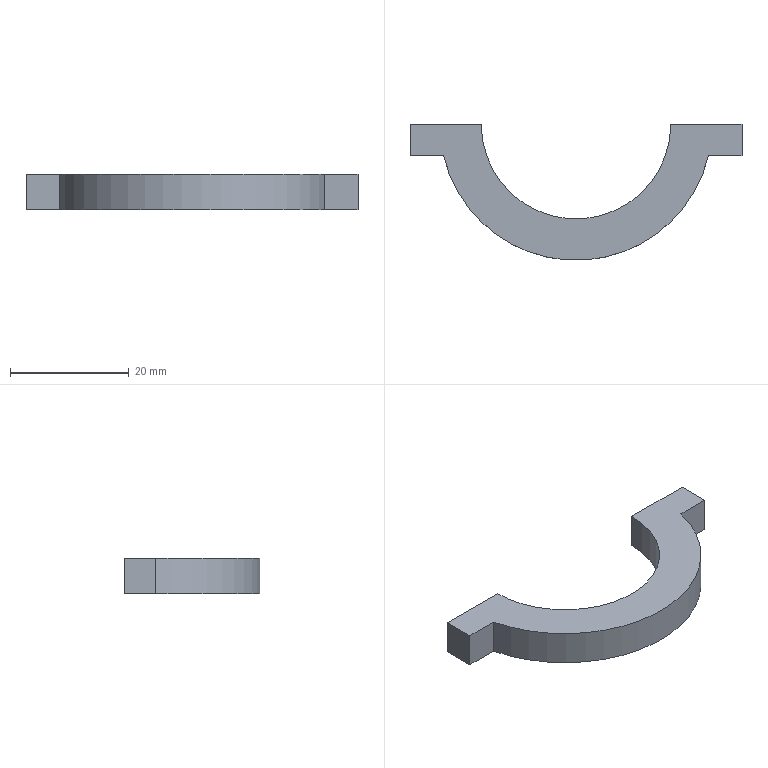Part | SolidWorks | features Extrusion 1 | 1 solid | 10 faces | box 56 x 22.979 x 6 mm | volume 2901 mm3 | plane 8 | cylinder 2 | commonest cylinder face diameters 32 x1 45.958 x1
STEP:
#1=CARTESIAN_POINT('',(16.,50.,0.));
#2=VERTEX_POINT('',#1);
#3=CARTESIAN_POINT('',(-16.,50.,0.));
#4=VERTEX_POINT('',#3);
#5=CARTESIAN_POINT('',(0.,50.,0.));
#6=DIRECTION('',(0.,0.,-1.));
#7=DIRECTION('',(1.,0.,0.));
#8=AXIS2_PLACEMENT_3D('',#5,#6,#7);
#9=CIRCLE('',#8,16.);
#10=EDGE_CURVE('',#2,#4,#9,.T.);
#11=ORIENTED_EDGE('',*,*,#10,.T.);
#12=CARTESIAN_POINT('',(-16.,50.,6.));
#13=VERTEX_POINT('',#12);
#14=CARTESIAN_POINT('',(-16.,50.,6.));
#15=DIRECTION('',(0.,0.,-1.));
#16=VECTOR('',#15,1000.);
#17=LINE('',#14,#16);
#18=EDGE_CURVE('',#13,#4,#17,.T.);
#19=ORIENTED_EDGE('',*,*,#18,.F.);
#20=CARTESIAN_POINT('',(16.,50.,6.));
#21=VERTEX_POINT('',#20);
#22=CARTESIAN_POINT('',(0.,50.,6.));
#23=DIRECTION('',(0.,0.,-1.));
#24=DIRECTION('',(1.,0.,0.));
#25=AXIS2_PLACEMENT_3D('',#22,#23,#24);
#26=CIRCLE('',#25,16.);
#27=EDGE_CURVE('',#21,#13,#26,.T.);
#28=ORIENTED_EDGE('',*,*,#27,.F.);
#29=CARTESIAN_POINT('',(16.,50.,6.));
#30=DIRECTION('',(0.,0.,-1.));
#31=VECTOR('',#30,1000.);
#32=LINE('',#29,#31);
#33=EDGE_CURVE('',#21,#2,#32,.T.);
#34=ORIENTED_EDGE('',*,*,#33,.T.);
#35=EDGE_LOOP('',(#11,#19,#28,#34));
#36=FACE_OUTER_BOUND('',#35,.T.);
#37=CARTESIAN_POINT('',(0.,50.,6.));
#38=DIRECTION('',(0.,0.,-1.));
#39=DIRECTION('',(-1.,0.,0.));
#40=AXIS2_PLACEMENT_3D('',#37,#38,#39);
#41=CYLINDRICAL_SURFACE('',#40,16.);
#42=ADVANCED_FACE('',(#36),#41,.F.);
#43=CARTESIAN_POINT('',(-28.,50.,0.));
#44=VERTEX_POINT('',#43);
#45=CARTESIAN_POINT('',(-16.,50.,0.));
#46=DIRECTION('',(-1.,0.,0.));
#47=VECTOR('',#46,1000.);
#48=LINE('',#45,#47);
#49=EDGE_CURVE('',#4,#44,#48,.T.);
#50=ORIENTED_EDGE('',*,*,#49,.T.);
#51=CARTESIAN_POINT('',(-28.,50.,6.));
#52=VERTEX_POINT('',#51);
#53=CARTESIAN_POINT('',(-28.,50.,6.));
#54=DIRECTION('',(0.,0.,-1.));
#55=VECTOR('',#54,1000.);
#56=LINE('',#53,#55);
#57=EDGE_CURVE('',#52,#44,#56,.T.);
#58=ORIENTED_EDGE('',*,*,#57,.F.);
#59=CARTESIAN_POINT('',(-16.,50.,6.));
#60=DIRECTION('',(-1.,0.,0.));
#61=VECTOR('',#60,1000.);
#62=LINE('',#59,#61);
#63=EDGE_CURVE('',#13,#52,#62,.T.);
#64=ORIENTED_EDGE('',*,*,#63,.F.);
#65=ORIENTED_EDGE('',*,*,#18,.T.);
#66=EDGE_LOOP('',(#50,#58,#64,#65));
#67=FACE_OUTER_BOUND('',#66,.T.);
#68=CARTESIAN_POINT('',(-16.,50.,6.));
#69=DIRECTION('',(0.,-1.,0.));
#70=DIRECTION('',(0.,0.,-1.));
#71=AXIS2_PLACEMENT_3D('',#68,#69,#70);
#72=PLANE('',#71);
#73=ADVANCED_FACE('',(#67),#72,.F.);
#74=CARTESIAN_POINT('',(-28.,44.637,0.));
#75=VERTEX_POINT('',#74);
#76=CARTESIAN_POINT('',(-28.,50.,0.));
#77=DIRECTION('',(0.,-1.,0.));
#78=VECTOR('',#77,1000.);
#79=LINE('',#76,#78);
#80=EDGE_CURVE('',#44,#75,#79,.T.);
#81=ORIENTED_EDGE('',*,*,#80,.T.);
#82=CARTESIAN_POINT('',(-28.,44.637,6.));
#83=VERTEX_POINT('',#82);
#84=CARTESIAN_POINT('',(-28.,44.637,6.));
#85=DIRECTION('',(0.,0.,-1.));
#86=VECTOR('',#85,1000.);
#87=LINE('',#84,#86);
#88=EDGE_CURVE('',#83,#75,#87,.T.);
#89=ORIENTED_EDGE('',*,*,#88,.F.);
#90=CARTESIAN_POINT('',(-28.,50.,6.));
#91=DIRECTION('',(0.,-1.,0.));
#92=VECTOR('',#91,1000.);
#93=LINE('',#90,#92);
#94=EDGE_CURVE('',#52,#83,#93,.T.);
#95=ORIENTED_EDGE('',*,*,#94,.F.);
#96=ORIENTED_EDGE('',*,*,#57,.T.);
#97=EDGE_LOOP('',(#81,#89,#95,#96));
#98=FACE_OUTER_BOUND('',#97,.T.);
#99=CARTESIAN_POINT('',(-28.,50.,6.));
#100=DIRECTION('',(1.,0.,0.));
#101=DIRECTION('',(0.,0.,-1.));
#102=AXIS2_PLACEMENT_3D('',#99,#100,#101);
#103=PLANE('',#102);
#104=ADVANCED_FACE('',(#98),#103,.F.);
#105=CARTESIAN_POINT('',(-22.345,44.637,0.));
#106=VERTEX_POINT('',#105);
#107=CARTESIAN_POINT('',(-22.345,44.637,0.));
#108=DIRECTION('',(1.,0.,0.));
#109=VECTOR('',#108,1000.);
#110=LINE('',#107,#109);
#111=EDGE_CURVE('',#75,#106,#110,.T.);
#112=ORIENTED_EDGE('',*,*,#111,.T.);
#113=CARTESIAN_POINT('',(-22.345,44.637,6.));
#114=VERTEX_POINT('',#113);
#115=CARTESIAN_POINT('',(-22.345,44.637,6.));
#116=DIRECTION('',(0.,0.,-1.));
#117=VECTOR('',#116,1000.);
#118=LINE('',#115,#117);
#119=EDGE_CURVE('',#114,#106,#118,.T.);
#120=ORIENTED_EDGE('',*,*,#119,.F.);
#121=CARTESIAN_POINT('',(-22.345,44.637,6.));
#122=DIRECTION('',(1.,0.,0.));
#123=VECTOR('',#122,1000.);
#124=LINE('',#121,#123);
#125=EDGE_CURVE('',#83,#114,#124,.T.);
#126=ORIENTED_EDGE('',*,*,#125,.F.);
#127=ORIENTED_EDGE('',*,*,#88,.T.);
#128=EDGE_LOOP('',(#112,#120,#126,#127));
#129=FACE_OUTER_BOUND('',#128,.T.);
#130=CARTESIAN_POINT('',(-22.345,44.637,6.));
#131=DIRECTION('',(0.,1.,0.));
#132=DIRECTION('',(0.,0.,1.));
#133=AXIS2_PLACEMENT_3D('',#130,#131,#132);
#134=PLANE('',#133);
#135=ADVANCED_FACE('',(#129),#134,.F.);
#136=CARTESIAN_POINT('',(22.345,44.637,0.));
#137=VERTEX_POINT('',#136);
#138=CARTESIAN_POINT('',(0.,50.,0.));
#139=DIRECTION('',(0.,0.,1.));
#140=DIRECTION('',(1.,0.,0.));
#141=AXIS2_PLACEMENT_3D('',#138,#139,#140);
#142=CIRCLE('',#141,22.979);
#143=EDGE_CURVE('',#106,#137,#142,.T.);
#144=ORIENTED_EDGE('',*,*,#143,.T.);
#145=CARTESIAN_POINT('',(22.345,44.637,6.));
#146=VERTEX_POINT('',#145);
#147=CARTESIAN_POINT('',(22.345,44.637,6.));
#148=DIRECTION('',(0.,0.,-1.));
#149=VECTOR('',#148,1000.);
#150=LINE('',#147,#149);
#151=EDGE_CURVE('',#146,#137,#150,.T.);
#152=ORIENTED_EDGE('',*,*,#151,.F.);
#153=CARTESIAN_POINT('',(0.,50.,6.));
#154=DIRECTION('',(0.,0.,1.));
#155=DIRECTION('',(1.,0.,0.));
#156=AXIS2_PLACEMENT_3D('',#153,#154,#155);
#157=CIRCLE('',#156,22.979);
#158=EDGE_CURVE('',#114,#146,#157,.T.);
#159=ORIENTED_EDGE('',*,*,#158,.F.);
#160=ORIENTED_EDGE('',*,*,#119,.T.);
#161=EDGE_LOOP('',(#144,#152,#159,#160));
#162=FACE_OUTER_BOUND('',#161,.T.);
#163=CARTESIAN_POINT('',(0.,50.,6.));
#164=DIRECTION('',(0.,0.,-1.));
#165=DIRECTION('',(-1.,0.,0.));
#166=AXIS2_PLACEMENT_3D('',#163,#164,#165);
#167=CYLINDRICAL_SURFACE('',#166,22.979);
#168=ADVANCED_FACE('',(#162),#167,.T.);
#169=CARTESIAN_POINT('',(28.,44.637,0.));
#170=VERTEX_POINT('',#169);
#171=CARTESIAN_POINT('',(28.,44.637,0.));
#172=DIRECTION('',(1.,0.,0.));
#173=VECTOR('',#172,1000.);
#174=LINE('',#171,#173);
#175=EDGE_CURVE('',#137,#170,#174,.T.);
#176=ORIENTED_EDGE('',*,*,#175,.T.);
#177=CARTESIAN_POINT('',(28.,44.637,6.));
#178=VERTEX_POINT('',#177);
#179=CARTESIAN_POINT('',(28.,44.637,6.));
#180=DIRECTION('',(0.,0.,-1.));
#181=VECTOR('',#180,1000.);
#182=LINE('',#179,#181);
#183=EDGE_CURVE('',#178,#170,#182,.T.);
#184=ORIENTED_EDGE('',*,*,#183,.F.);
#185=CARTESIAN_POINT('',(28.,44.637,6.));
#186=DIRECTION('',(1.,0.,0.));
#187=VECTOR('',#186,1000.);
#188=LINE('',#185,#187);
#189=EDGE_CURVE('',#146,#178,#188,.T.);
#190=ORIENTED_EDGE('',*,*,#189,.F.);
#191=ORIENTED_EDGE('',*,*,#151,.T.);
#192=EDGE_LOOP('',(#176,#184,#190,#191));
#193=FACE_OUTER_BOUND('',#192,.T.);
#194=CARTESIAN_POINT('',(28.,44.637,6.));
#195=DIRECTION('',(0.,1.,0.));
#196=DIRECTION('',(0.,0.,1.));
#197=AXIS2_PLACEMENT_3D('',#194,#195,#196);
#198=PLANE('',#197);
#199=ADVANCED_FACE('',(#193),#198,.F.);
#200=CARTESIAN_POINT('',(28.,50.,0.));
#201=VERTEX_POINT('',#200);
#202=CARTESIAN_POINT('',(28.,50.,0.));
#203=DIRECTION('',(0.,1.,0.));
#204=VECTOR('',#203,1000.);
#205=LINE('',#202,#204);
#206=EDGE_CURVE('',#170,#201,#205,.T.);
#207=ORIENTED_EDGE('',*,*,#206,.T.);
#208=CARTESIAN_POINT('',(28.,50.,6.));
#209=VERTEX_POINT('',#208);
#210=CARTESIAN_POINT('',(28.,50.,6.));
#211=DIRECTION('',(0.,0.,-1.));
#212=VECTOR('',#211,1000.);
#213=LINE('',#210,#212);
#214=EDGE_CURVE('',#209,#201,#213,.T.);
#215=ORIENTED_EDGE('',*,*,#214,.F.);
#216=CARTESIAN_POINT('',(28.,50.,6.));
#217=DIRECTION('',(0.,1.,0.));
#218=VECTOR('',#217,1000.);
#219=LINE('',#216,#218);
#220=EDGE_CURVE('',#178,#209,#219,.T.);
#221=ORIENTED_EDGE('',*,*,#220,.F.);
#222=ORIENTED_EDGE('',*,*,#183,.T.);
#223=EDGE_LOOP('',(#207,#215,#221,#222));
#224=FACE_OUTER_BOUND('',#223,.T.);
#225=CARTESIAN_POINT('',(28.,50.,6.));
#226=DIRECTION('',(-1.,0.,0.));
#227=DIRECTION('',(0.,0.,1.));
#228=AXIS2_PLACEMENT_3D('',#225,#226,#227);
#229=PLANE('',#228);
#230=ADVANCED_FACE('',(#224),#229,.F.);
#231=CARTESIAN_POINT('',(16.,50.,0.));
#232=DIRECTION('',(-1.,0.,0.));
#233=VECTOR('',#232,1000.);
#234=LINE('',#231,#233);
#235=EDGE_CURVE('',#201,#2,#234,.T.);
#236=ORIENTED_EDGE('',*,*,#235,.T.);
#237=ORIENTED_EDGE('',*,*,#33,.F.);
#238=CARTESIAN_POINT('',(16.,50.,6.));
#239=DIRECTION('',(-1.,0.,0.));
#240=VECTOR('',#239,1000.);
#241=LINE('',#238,#240);
#242=EDGE_CURVE('',#209,#21,#241,.T.);
#243=ORIENTED_EDGE('',*,*,#242,.F.);
#244=ORIENTED_EDGE('',*,*,#214,.T.);
#245=EDGE_LOOP('',(#236,#237,#243,#244));
#246=FACE_OUTER_BOUND('',#245,.T.);
#247=CARTESIAN_POINT('',(16.,50.,6.));
#248=DIRECTION('',(0.,-1.,0.));
#249=DIRECTION('',(0.,0.,-1.));
#250=AXIS2_PLACEMENT_3D('',#247,#248,#249);
#251=PLANE('',#250);
#252=ADVANCED_FACE('',(#246),#251,.F.);
#253=ORIENTED_EDGE('',*,*,#27,.T.);
#254=ORIENTED_EDGE('',*,*,#63,.T.);
#255=ORIENTED_EDGE('',*,*,#94,.T.);
#256=ORIENTED_EDGE('',*,*,#125,.T.);
#257=ORIENTED_EDGE('',*,*,#158,.T.);
#258=ORIENTED_EDGE('',*,*,#189,.T.);
#259=ORIENTED_EDGE('',*,*,#220,.T.);
#260=ORIENTED_EDGE('',*,*,#242,.T.);
#261=EDGE_LOOP('',(#253,#254,#255,#256,#257,#258,#259,#260));
#262=FACE_OUTER_BOUND('',#261,.T.);
#263=CARTESIAN_POINT('',(0.,50.,6.));
#264=DIRECTION('',(0.,0.,1.));
#265=DIRECTION('',(1.,0.,0.));
#266=AXIS2_PLACEMENT_3D('',#263,#264,#265);
#267=PLANE('',#266);
#268=ADVANCED_FACE('',(#262),#267,.T.);
#269=ORIENTED_EDGE('',*,*,#10,.F.);
#270=ORIENTED_EDGE('',*,*,#235,.F.);
#271=ORIENTED_EDGE('',*,*,#206,.F.);
#272=ORIENTED_EDGE('',*,*,#175,.F.);
#273=ORIENTED_EDGE('',*,*,#143,.F.);
#274=ORIENTED_EDGE('',*,*,#111,.F.);
#275=ORIENTED_EDGE('',*,*,#80,.F.);
#276=ORIENTED_EDGE('',*,*,#49,.F.);
#277=EDGE_LOOP('',(#269,#270,#271,#272,#273,#274,#275,#276));
#278=FACE_OUTER_BOUND('',#277,.T.);
#279=CARTESIAN_POINT('',(0.,50.,0.));
#280=DIRECTION('',(0.,0.,1.));
#281=DIRECTION('',(1.,0.,0.));
#282=AXIS2_PLACEMENT_3D('',#279,#280,#281);
#283=PLANE('',#282);
#284=ADVANCED_FACE('',(#278),#283,.F.);
#285=CLOSED_SHELL('',(#42,#73,#104,#135,#168,#199,#230,#252,#268,#284));
#286=MANIFOLD_SOLID_BREP('',#285);
#287=CARTESIAN_POINT('',(0.,0.,0.));
#288=DIRECTION('',(0.,0.,1.));
#289=DIRECTION('',(1.,0.,0.));
#290=AXIS2_PLACEMENT_3D('',#287,#288,#289);
#291=(LENGTH_UNIT()NAMED_UNIT(*)SI_UNIT(.MILLI.,.METRE.));
#292=UNCERTAINTY_MEASURE_WITH_UNIT(LENGTH_MEASURE(0.00001),#291,'','');
#293=(NAMED_UNIT(*)PLANE_ANGLE_UNIT()SI_UNIT($,.RADIAN.));
#294=(NAMED_UNIT(*)SI_UNIT($,.STERADIAN.)SOLID_ANGLE_UNIT());
#295=(GEOMETRIC_REPRESENTATION_CONTEXT(3)GLOBAL_UNCERTAINTY_ASSIGNED_CONTEXT((#292))GLOBAL_UNIT_ASSIGNED_CONTEXT((#291,#293,#294))REPRESENTATION_CONTEXT('',''));
#296=ADVANCED_BREP_SHAPE_REPRESENTATION('',(#286,#290),#295);